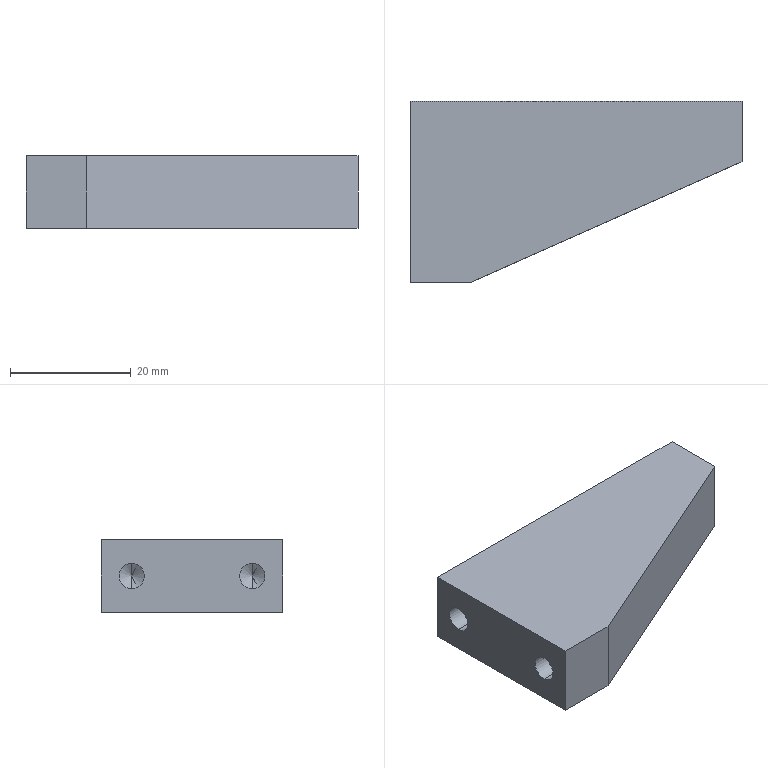Part | SolidWorks | features 3DProfileFeature 2, HoleWzd 2, Extrusion 1 | 1 solid | 23 faces | box 55 x 30 x 12 mm | volume 13823 mm3 | cylinder 8 | cone 8 | plane 7 | commonest cylinder face diameters 4.2 x8
STEP:
#1=CARTESIAN_POINT('',(-30.107,9.119,3.9));
#2=VERTEX_POINT('',#1);
#3=CARTESIAN_POINT('',(-30.107,9.119,8.1));
#4=VERTEX_POINT('',#3);
#5=CARTESIAN_POINT('',(-30.107,9.119,6.));
#6=DIRECTION('',(-1.,0.,0.));
#7=DIRECTION('',(0.,0.,1.));
#8=AXIS2_PLACEMENT_3D('',#5,#6,#7);
#9=CIRCLE('',#8,2.1);
#10=EDGE_CURVE('',#2,#4,#9,.T.);
#11=ORIENTED_EDGE('',*,*,#10,.F.);
#12=CARTESIAN_POINT('',(-40.107,9.119,3.9));
#13=VERTEX_POINT('',#12);
#14=CARTESIAN_POINT('',(-40.107,9.119,3.9));
#15=DIRECTION('',(-1.,0.,0.));
#16=VECTOR('',#15,1000.);
#17=LINE('',#14,#16);
#18=EDGE_CURVE('',#2,#13,#17,.T.);
#19=ORIENTED_EDGE('',*,*,#18,.T.);
#20=CARTESIAN_POINT('',(-40.107,9.119,8.1));
#21=VERTEX_POINT('',#20);
#22=CARTESIAN_POINT('',(-40.107,9.119,6.));
#23=DIRECTION('',(-1.,0.,0.));
#24=DIRECTION('',(0.,0.,1.));
#25=AXIS2_PLACEMENT_3D('',#22,#23,#24);
#26=CIRCLE('',#25,2.1);
#27=EDGE_CURVE('',#13,#21,#26,.T.);
#28=ORIENTED_EDGE('',*,*,#27,.T.);
#29=CARTESIAN_POINT('',(-40.107,9.119,8.1));
#30=DIRECTION('',(-1.,0.,0.));
#31=VECTOR('',#30,1000.);
#32=LINE('',#29,#31);
#33=EDGE_CURVE('',#4,#21,#32,.T.);
#34=ORIENTED_EDGE('',*,*,#33,.F.);
#35=EDGE_LOOP('',(#11,#19,#28,#34));
#36=FACE_OUTER_BOUND('',#35,.T.);
#37=CARTESIAN_POINT('',(-40.107,9.119,6.));
#38=DIRECTION('',(-1.,0.,0.));
#39=DIRECTION('',(0.,0.,1.));
#40=AXIS2_PLACEMENT_3D('',#37,#38,#39);
#41=CYLINDRICAL_SURFACE('',#40,2.1);
#42=ADVANCED_FACE('',(#36),#41,.F.);
#43=CARTESIAN_POINT('',(-28.845,9.119,6.));
#44=VERTEX_POINT('',#43);
#45=CARTESIAN_POINT('',(-30.107,9.119,8.1));
#46=DIRECTION('',(-0.515,0.,0.8572));
#47=VECTOR('',#46,1000.);
#48=LINE('',#45,#47);
#49=EDGE_CURVE('',#44,#4,#48,.T.);
#50=ORIENTED_EDGE('',*,*,#49,.F.);
#51=CARTESIAN_POINT('',(-30.107,9.119,3.9));
#52=DIRECTION('',(-0.515,0.,-0.8572));
#53=VECTOR('',#52,1000.);
#54=LINE('',#51,#53);
#55=EDGE_CURVE('',#44,#2,#54,.T.);
#56=ORIENTED_EDGE('',*,*,#55,.T.);
#57=ORIENTED_EDGE('',*,*,#10,.T.);
#58=EDGE_LOOP('',(#50,#56,#57));
#59=FACE_OUTER_BOUND('',#58,.T.);
#60=CARTESIAN_POINT('',(-30.107,9.119,6.));
#61=DIRECTION('',(-1.,0.,0.));
#62=DIRECTION('',(0.,0.,1.));
#63=AXIS2_PLACEMENT_3D('',#60,#61,#62);
#64=CONICAL_SURFACE('',#63,2.1,1.03);
#65=ADVANCED_FACE('',(#59),#64,.F.);
#66=CARTESIAN_POINT('',(-30.107,29.119,3.9));
#67=VERTEX_POINT('',#66);
#68=CARTESIAN_POINT('',(-30.107,29.119,8.1));
#69=VERTEX_POINT('',#68);
#70=CARTESIAN_POINT('',(-30.107,29.119,6.));
#71=DIRECTION('',(-1.,0.,0.));
#72=DIRECTION('',(0.,0.,1.));
#73=AXIS2_PLACEMENT_3D('',#70,#71,#72);
#74=CIRCLE('',#73,2.1);
#75=EDGE_CURVE('',#67,#69,#74,.T.);
#76=ORIENTED_EDGE('',*,*,#75,.F.);
#77=CARTESIAN_POINT('',(-40.107,29.119,3.9));
#78=VERTEX_POINT('',#77);
#79=CARTESIAN_POINT('',(-40.107,29.119,3.9));
#80=DIRECTION('',(-1.,0.,0.));
#81=VECTOR('',#80,1000.);
#82=LINE('',#79,#81);
#83=EDGE_CURVE('',#67,#78,#82,.T.);
#84=ORIENTED_EDGE('',*,*,#83,.T.);
#85=CARTESIAN_POINT('',(-40.107,29.119,8.1));
#86=VERTEX_POINT('',#85);
#87=CARTESIAN_POINT('',(-40.107,29.119,6.));
#88=DIRECTION('',(-1.,0.,0.));
#89=DIRECTION('',(0.,0.,1.));
#90=AXIS2_PLACEMENT_3D('',#87,#88,#89);
#91=CIRCLE('',#90,2.1);
#92=EDGE_CURVE('',#78,#86,#91,.T.);
#93=ORIENTED_EDGE('',*,*,#92,.T.);
#94=CARTESIAN_POINT('',(-40.107,29.119,8.1));
#95=DIRECTION('',(-1.,0.,0.));
#96=VECTOR('',#95,1000.);
#97=LINE('',#94,#96);
#98=EDGE_CURVE('',#69,#86,#97,.T.);
#99=ORIENTED_EDGE('',*,*,#98,.F.);
#100=EDGE_LOOP('',(#76,#84,#93,#99));
#101=FACE_OUTER_BOUND('',#100,.T.);
#102=CARTESIAN_POINT('',(-40.107,29.119,6.));
#103=DIRECTION('',(-1.,0.,0.));
#104=DIRECTION('',(0.,0.,1.));
#105=AXIS2_PLACEMENT_3D('',#102,#103,#104);
#106=CYLINDRICAL_SURFACE('',#105,2.1);
#107=ADVANCED_FACE('',(#101),#106,.F.);
#108=CARTESIAN_POINT('',(-28.845,29.119,6.));
#109=VERTEX_POINT('',#108);
#110=CARTESIAN_POINT('',(-30.107,29.119,8.1));
#111=DIRECTION('',(-0.515,0.,0.8572));
#112=VECTOR('',#111,1000.);
#113=LINE('',#110,#112);
#114=EDGE_CURVE('',#109,#69,#113,.T.);
#115=ORIENTED_EDGE('',*,*,#114,.F.);
#116=CARTESIAN_POINT('',(-30.107,29.119,3.9));
#117=DIRECTION('',(-0.515,0.,-0.8572));
#118=VECTOR('',#117,1000.);
#119=LINE('',#116,#118);
#120=EDGE_CURVE('',#109,#67,#119,.T.);
#121=ORIENTED_EDGE('',*,*,#120,.T.);
#122=ORIENTED_EDGE('',*,*,#75,.T.);
#123=EDGE_LOOP('',(#115,#121,#122));
#124=FACE_OUTER_BOUND('',#123,.T.);
#125=CARTESIAN_POINT('',(-30.107,29.119,6.));
#126=DIRECTION('',(-1.,0.,0.));
#127=DIRECTION('',(0.,0.,1.));
#128=AXIS2_PLACEMENT_3D('',#125,#126,#127);
#129=CONICAL_SURFACE('',#128,2.1,1.03);
#130=ADVANCED_FACE('',(#124),#129,.F.);
#131=CARTESIAN_POINT('',(-24.107,24.119,3.9));
#132=VERTEX_POINT('',#131);
#133=CARTESIAN_POINT('',(-24.107,24.119,8.1));
#134=VERTEX_POINT('',#133);
#135=CARTESIAN_POINT('',(-24.107,24.119,6.));
#136=DIRECTION('',(0.,1.,0.));
#137=DIRECTION('',(0.,0.,1.));
#138=AXIS2_PLACEMENT_3D('',#135,#136,#137);
#139=CIRCLE('',#138,2.1);
#140=EDGE_CURVE('',#132,#134,#139,.T.);
#141=ORIENTED_EDGE('',*,*,#140,.F.);
#142=CARTESIAN_POINT('',(-24.107,34.119,3.9));
#143=VERTEX_POINT('',#142);
#144=CARTESIAN_POINT('',(-24.107,34.119,3.9));
#145=DIRECTION('',(0.,1.,0.));
#146=VECTOR('',#145,1000.);
#147=LINE('',#144,#146);
#148=EDGE_CURVE('',#132,#143,#147,.T.);
#149=ORIENTED_EDGE('',*,*,#148,.T.);
#150=CARTESIAN_POINT('',(-24.107,34.119,8.1));
#151=VERTEX_POINT('',#150);
#152=CARTESIAN_POINT('',(-24.107,34.119,6.));
#153=DIRECTION('',(0.,1.,0.));
#154=DIRECTION('',(0.,0.,1.));
#155=AXIS2_PLACEMENT_3D('',#152,#153,#154);
#156=CIRCLE('',#155,2.1);
#157=EDGE_CURVE('',#143,#151,#156,.T.);
#158=ORIENTED_EDGE('',*,*,#157,.T.);
#159=CARTESIAN_POINT('',(-24.107,34.119,8.1));
#160=DIRECTION('',(0.,1.,0.));
#161=VECTOR('',#160,1000.);
#162=LINE('',#159,#161);
#163=EDGE_CURVE('',#134,#151,#162,.T.);
#164=ORIENTED_EDGE('',*,*,#163,.F.);
#165=EDGE_LOOP('',(#141,#149,#158,#164));
#166=FACE_OUTER_BOUND('',#165,.T.);
#167=CARTESIAN_POINT('',(-24.107,34.119,6.));
#168=DIRECTION('',(0.,1.,0.));
#169=DIRECTION('',(0.,0.,1.));
#170=AXIS2_PLACEMENT_3D('',#167,#168,#169);
#171=CYLINDRICAL_SURFACE('',#170,2.1);
#172=ADVANCED_FACE('',(#166),#171,.F.);
#173=CARTESIAN_POINT('',(-24.107,22.857,6.));
#174=VERTEX_POINT('',#173);
#175=CARTESIAN_POINT('',(-24.107,24.119,8.1));
#176=DIRECTION('',(0.,0.515,0.8572));
#177=VECTOR('',#176,1000.);
#178=LINE('',#175,#177);
#179=EDGE_CURVE('',#174,#134,#178,.T.);
#180=ORIENTED_EDGE('',*,*,#179,.F.);
#181=CARTESIAN_POINT('',(-24.107,24.119,3.9));
#182=DIRECTION('',(0.,0.515,-0.8572));
#183=VECTOR('',#182,1000.);
#184=LINE('',#181,#183);
#185=EDGE_CURVE('',#174,#132,#184,.T.);
#186=ORIENTED_EDGE('',*,*,#185,.T.);
#187=ORIENTED_EDGE('',*,*,#140,.T.);
#188=EDGE_LOOP('',(#180,#186,#187));
#189=FACE_OUTER_BOUND('',#188,.T.);
#190=CARTESIAN_POINT('',(-24.107,24.119,6.));
#191=DIRECTION('',(0.,1.,0.));
#192=DIRECTION('',(0.,0.,1.));
#193=AXIS2_PLACEMENT_3D('',#190,#191,#192);
#194=CONICAL_SURFACE('',#193,2.1,1.03);
#195=ADVANCED_FACE('',(#189),#194,.F.);
#196=CARTESIAN_POINT('',(5.893,24.119,3.9));
#197=VERTEX_POINT('',#196);
#198=CARTESIAN_POINT('',(5.893,24.119,8.1));
#199=VERTEX_POINT('',#198);
#200=CARTESIAN_POINT('',(5.893,24.119,6.));
#201=DIRECTION('',(0.,1.,0.));
#202=DIRECTION('',(0.,0.,1.));
#203=AXIS2_PLACEMENT_3D('',#200,#201,#202);
#204=CIRCLE('',#203,2.1);
#205=EDGE_CURVE('',#197,#199,#204,.T.);
#206=ORIENTED_EDGE('',*,*,#205,.F.);
#207=CARTESIAN_POINT('',(5.893,34.119,3.9));
#208=VERTEX_POINT('',#207);
#209=CARTESIAN_POINT('',(5.893,34.119,3.9));
#210=DIRECTION('',(0.,1.,0.));
#211=VECTOR('',#210,1000.);
#212=LINE('',#209,#211);
#213=EDGE_CURVE('',#197,#208,#212,.T.);
#214=ORIENTED_EDGE('',*,*,#213,.T.);
#215=CARTESIAN_POINT('',(5.893,34.119,8.1));
#216=VERTEX_POINT('',#215);
#217=CARTESIAN_POINT('',(5.893,34.119,6.));
#218=DIRECTION('',(0.,1.,0.));
#219=DIRECTION('',(0.,0.,1.));
#220=AXIS2_PLACEMENT_3D('',#217,#218,#219);
#221=CIRCLE('',#220,2.1);
#222=EDGE_CURVE('',#208,#216,#221,.T.);
#223=ORIENTED_EDGE('',*,*,#222,.T.);
#224=CARTESIAN_POINT('',(5.893,34.119,8.1));
#225=DIRECTION('',(0.,1.,0.));
#226=VECTOR('',#225,1000.);
#227=LINE('',#224,#226);
#228=EDGE_CURVE('',#199,#216,#227,.T.);
#229=ORIENTED_EDGE('',*,*,#228,.F.);
#230=EDGE_LOOP('',(#206,#214,#223,#229));
#231=FACE_OUTER_BOUND('',#230,.T.);
#232=CARTESIAN_POINT('',(5.893,34.119,6.));
#233=DIRECTION('',(0.,1.,0.));
#234=DIRECTION('',(0.,0.,1.));
#235=AXIS2_PLACEMENT_3D('',#232,#233,#234);
#236=CYLINDRICAL_SURFACE('',#235,2.1);
#237=ADVANCED_FACE('',(#231),#236,.F.);
#238=CARTESIAN_POINT('',(5.893,22.857,6.));
#239=VERTEX_POINT('',#238);
#240=CARTESIAN_POINT('',(5.893,24.119,8.1));
#241=DIRECTION('',(0.,0.515,0.8572));
#242=VECTOR('',#241,1000.);
#243=LINE('',#240,#242);
#244=EDGE_CURVE('',#239,#199,#243,.T.);
#245=ORIENTED_EDGE('',*,*,#244,.F.);
#246=CARTESIAN_POINT('',(5.893,24.119,3.9));
#247=DIRECTION('',(0.,0.515,-0.8572));
#248=VECTOR('',#247,1000.);
#249=LINE('',#246,#248);
#250=EDGE_CURVE('',#239,#197,#249,.T.);
#251=ORIENTED_EDGE('',*,*,#250,.T.);
#252=ORIENTED_EDGE('',*,*,#205,.T.);
#253=EDGE_LOOP('',(#245,#251,#252));
#254=FACE_OUTER_BOUND('',#253,.T.);
#255=CARTESIAN_POINT('',(5.893,24.119,6.));
#256=DIRECTION('',(0.,1.,0.));
#257=DIRECTION('',(0.,0.,1.));
#258=AXIS2_PLACEMENT_3D('',#255,#256,#257);
#259=CONICAL_SURFACE('',#258,2.1,1.03);
#260=ADVANCED_FACE('',(#254),#259,.F.);
#261=CARTESIAN_POINT('',(-30.107,4.119,0.));
#262=VERTEX_POINT('',#261);
#263=CARTESIAN_POINT('',(14.893,24.119,0.));
#264=VERTEX_POINT('',#263);
#265=CARTESIAN_POINT('',(14.893,24.119,0.));
#266=DIRECTION('',(0.9138,0.4061,0.));
#267=VECTOR('',#266,1000.);
#268=LINE('',#265,#267);
#269=EDGE_CURVE('',#262,#264,#268,.T.);
#270=ORIENTED_EDGE('',*,*,#269,.T.);
#271=CARTESIAN_POINT('',(14.893,24.119,12.));
#272=VERTEX_POINT('',#271);
#273=CARTESIAN_POINT('',(14.893,24.119,12.));
#274=DIRECTION('',(0.,0.,-1.));
#275=VECTOR('',#274,1000.);
#276=LINE('',#273,#275);
#277=EDGE_CURVE('',#272,#264,#276,.T.);
#278=ORIENTED_EDGE('',*,*,#277,.F.);
#279=CARTESIAN_POINT('',(-30.107,4.119,12.));
#280=VERTEX_POINT('',#279);
#281=CARTESIAN_POINT('',(14.893,24.119,12.));
#282=DIRECTION('',(0.9138,0.4061,0.));
#283=VECTOR('',#282,1000.);
#284=LINE('',#281,#283);
#285=EDGE_CURVE('',#280,#272,#284,.T.);
#286=ORIENTED_EDGE('',*,*,#285,.F.);
#287=CARTESIAN_POINT('',(-30.107,4.119,12.));
#288=DIRECTION('',(0.,0.,-1.));
#289=VECTOR('',#288,1000.);
#290=LINE('',#287,#289);
#291=EDGE_CURVE('',#280,#262,#290,.T.);
#292=ORIENTED_EDGE('',*,*,#291,.T.);
#293=EDGE_LOOP('',(#270,#278,#286,#292));
#294=FACE_OUTER_BOUND('',#293,.T.);
#295=CARTESIAN_POINT('',(14.893,24.119,12.));
#296=DIRECTION('',(-0.4061,0.9138,0.));
#297=DIRECTION('',(-0.9138,-0.4061,0.));
#298=AXIS2_PLACEMENT_3D('',#295,#296,#297);
#299=PLANE('',#298);
#300=ADVANCED_FACE('',(#294),#299,.F.);
#301=CARTESIAN_POINT('',(14.893,34.119,0.));
#302=VERTEX_POINT('',#301);
#303=CARTESIAN_POINT('',(14.893,34.119,0.));
#304=DIRECTION('',(0.,1.,0.));
#305=VECTOR('',#304,1000.);
#306=LINE('',#303,#305);
#307=EDGE_CURVE('',#264,#302,#306,.T.);
#308=ORIENTED_EDGE('',*,*,#307,.T.);
#309=CARTESIAN_POINT('',(14.893,34.119,12.));
#310=VERTEX_POINT('',#309);
#311=CARTESIAN_POINT('',(14.893,34.119,12.));
#312=DIRECTION('',(0.,0.,-1.));
#313=VECTOR('',#312,1000.);
#314=LINE('',#311,#313);
#315=EDGE_CURVE('',#310,#302,#314,.T.);
#316=ORIENTED_EDGE('',*,*,#315,.F.);
#317=CARTESIAN_POINT('',(14.893,34.119,12.));
#318=DIRECTION('',(0.,1.,0.));
#319=VECTOR('',#318,1000.);
#320=LINE('',#317,#319);
#321=EDGE_CURVE('',#272,#310,#320,.T.);
#322=ORIENTED_EDGE('',*,*,#321,.F.);
#323=ORIENTED_EDGE('',*,*,#277,.T.);
#324=EDGE_LOOP('',(#308,#316,#322,#323));
#325=FACE_OUTER_BOUND('',#324,.T.);
#326=CARTESIAN_POINT('',(14.893,34.119,12.));
#327=DIRECTION('',(-1.,0.,0.));
#328=DIRECTION('',(0.,-1.,0.));
#329=AXIS2_PLACEMENT_3D('',#326,#327,#328);
#330=PLANE('',#329);
#331=ADVANCED_FACE('',(#325),#330,.F.);
#332=CARTESIAN_POINT('',(-24.107,34.119,6.));
#333=DIRECTION('',(0.,1.,0.));
#334=DIRECTION('',(0.,0.,1.));
#335=AXIS2_PLACEMENT_3D('',#332,#333,#334);
#336=CIRCLE('',#335,2.1);
#337=EDGE_CURVE('',#151,#143,#336,.T.);
#338=ORIENTED_EDGE('',*,*,#337,.F.);
#339=ORIENTED_EDGE('',*,*,#157,.F.);
#340=EDGE_LOOP('',(#338,#339));
#341=FACE_BOUND('',#340,.T.);
#342=CARTESIAN_POINT('',(5.893,34.119,6.));
#343=DIRECTION('',(0.,1.,0.));
#344=DIRECTION('',(0.,0.,1.));
#345=AXIS2_PLACEMENT_3D('',#342,#343,#344);
#346=CIRCLE('',#345,2.1);
#347=EDGE_CURVE('',#216,#208,#346,.T.);
#348=ORIENTED_EDGE('',*,*,#347,.F.);
#349=ORIENTED_EDGE('',*,*,#222,.F.);
#350=EDGE_LOOP('',(#348,#349));
#351=FACE_BOUND('',#350,.T.);
#352=CARTESIAN_POINT('',(-40.107,34.119,0.));
#353=VERTEX_POINT('',#352);
#354=CARTESIAN_POINT('',(-40.107,34.119,0.));
#355=DIRECTION('',(-1.,0.,0.));
#356=VECTOR('',#355,1000.);
#357=LINE('',#354,#356);
#358=EDGE_CURVE('',#302,#353,#357,.T.);
#359=ORIENTED_EDGE('',*,*,#358,.T.);
#360=CARTESIAN_POINT('',(-40.107,34.119,12.));
#361=VERTEX_POINT('',#360);
#362=CARTESIAN_POINT('',(-40.107,34.119,12.));
#363=DIRECTION('',(0.,0.,-1.));
#364=VECTOR('',#363,1000.);
#365=LINE('',#362,#364);
#366=EDGE_CURVE('',#361,#353,#365,.T.);
#367=ORIENTED_EDGE('',*,*,#366,.F.);
#368=CARTESIAN_POINT('',(-40.107,34.119,12.));
#369=DIRECTION('',(-1.,0.,0.));
#370=VECTOR('',#369,1000.);
#371=LINE('',#368,#370);
#372=EDGE_CURVE('',#310,#361,#371,.T.);
#373=ORIENTED_EDGE('',*,*,#372,.F.);
#374=ORIENTED_EDGE('',*,*,#315,.T.);
#375=EDGE_LOOP('',(#359,#367,#373,#374));
#376=FACE_OUTER_BOUND('',#375,.T.);
#377=CARTESIAN_POINT('',(-40.107,34.119,12.));
#378=DIRECTION('',(0.,-1.,0.));
#379=DIRECTION('',(0.,0.,-1.));
#380=AXIS2_PLACEMENT_3D('',#377,#378,#379);
#381=PLANE('',#380);
#382=ADVANCED_FACE('',(#341,#351,#376),#381,.F.);
#383=CARTESIAN_POINT('',(-40.107,9.119,6.));
#384=DIRECTION('',(-1.,0.,0.));
#385=DIRECTION('',(0.,0.,1.));
#386=AXIS2_PLACEMENT_3D('',#383,#384,#385);
#387=CIRCLE('',#386,2.1);
#388=EDGE_CURVE('',#21,#13,#387,.T.);
#389=ORIENTED_EDGE('',*,*,#388,.F.);
#390=ORIENTED_EDGE('',*,*,#27,.F.);
#391=EDGE_LOOP('',(#389,#390));
#392=FACE_BOUND('',#391,.T.);
#393=CARTESIAN_POINT('',(-40.107,29.119,6.));
#394=DIRECTION('',(-1.,0.,0.));
#395=DIRECTION('',(0.,0.,1.));
#396=AXIS2_PLACEMENT_3D('',#393,#394,#395);
#397=CIRCLE('',#396,2.1);
#398=EDGE_CURVE('',#86,#78,#397,.T.);
#399=ORIENTED_EDGE('',*,*,#398,.F.);
#400=ORIENTED_EDGE('',*,*,#92,.F.);
#401=EDGE_LOOP('',(#399,#400));
#402=FACE_BOUND('',#401,.T.);
#403=CARTESIAN_POINT('',(-40.107,4.119,0.));
#404=VERTEX_POINT('',#403);
#405=CARTESIAN_POINT('',(-40.107,4.119,0.));
#406=DIRECTION('',(0.,-1.,0.));
#407=VECTOR('',#406,1000.);
#408=LINE('',#405,#407);
#409=EDGE_CURVE('',#353,#404,#408,.T.);
#410=ORIENTED_EDGE('',*,*,#409,.T.);
#411=CARTESIAN_POINT('',(-40.107,4.119,12.));
#412=VERTEX_POINT('',#411);
#413=CARTESIAN_POINT('',(-40.107,4.119,12.));
#414=DIRECTION('',(0.,0.,-1.));
#415=VECTOR('',#414,1000.);
#416=LINE('',#413,#415);
#417=EDGE_CURVE('',#412,#404,#416,.T.);
#418=ORIENTED_EDGE('',*,*,#417,.F.);
#419=CARTESIAN_POINT('',(-40.107,4.119,12.));
#420=DIRECTION('',(0.,-1.,0.));
#421=VECTOR('',#420,1000.);
#422=LINE('',#419,#421);
#423=EDGE_CURVE('',#361,#412,#422,.T.);
#424=ORIENTED_EDGE('',*,*,#423,.F.);
#425=ORIENTED_EDGE('',*,*,#366,.T.);
#426=EDGE_LOOP('',(#410,#418,#424,#425));
#427=FACE_OUTER_BOUND('',#426,.T.);
#428=CARTESIAN_POINT('',(-40.107,4.119,12.));
#429=DIRECTION('',(1.,0.,0.));
#430=DIRECTION('',(0.,0.,-1.));
#431=AXIS2_PLACEMENT_3D('',#428,#429,#430);
#432=PLANE('',#431);
#433=ADVANCED_FACE('',(#392,#402,#427),#432,.F.);
#434=CARTESIAN_POINT('',(-30.107,4.119,0.));
#435=DIRECTION('',(1.,0.,0.));
#436=VECTOR('',#435,1000.);
#437=LINE('',#434,#436);
#438=EDGE_CURVE('',#404,#262,#437,.T.);
#439=ORIENTED_EDGE('',*,*,#438,.T.);
#440=ORIENTED_EDGE('',*,*,#291,.F.);
#441=CARTESIAN_POINT('',(-30.107,4.119,12.));
#442=DIRECTION('',(1.,0.,0.));
#443=VECTOR('',#442,1000.);
#444=LINE('',#441,#443);
#445=EDGE_CURVE('',#412,#280,#444,.T.);
#446=ORIENTED_EDGE('',*,*,#445,.F.);
#447=ORIENTED_EDGE('',*,*,#417,.T.);
#448=EDGE_LOOP('',(#439,#440,#446,#447));
#449=FACE_OUTER_BOUND('',#448,.T.);
#450=CARTESIAN_POINT('',(-30.107,4.119,12.));
#451=DIRECTION('',(0.,1.,0.));
#452=DIRECTION('',(-1.,0.,0.));
#453=AXIS2_PLACEMENT_3D('',#450,#451,#452);
#454=PLANE('',#453);
#455=ADVANCED_FACE('',(#449),#454,.F.);
#456=ORIENTED_EDGE('',*,*,#285,.T.);
#457=ORIENTED_EDGE('',*,*,#321,.T.);
#458=ORIENTED_EDGE('',*,*,#372,.T.);
#459=ORIENTED_EDGE('',*,*,#423,.T.);
#460=ORIENTED_EDGE('',*,*,#445,.T.);
#461=EDGE_LOOP('',(#456,#457,#458,#459,#460));
#462=FACE_OUTER_BOUND('',#461,.T.);
#463=CARTESIAN_POINT('',(-40.107,-0.3259,12.));
#464=DIRECTION('',(0.,0.,-1.));
#465=DIRECTION('',(-1.,0.,0.));
#466=AXIS2_PLACEMENT_3D('',#463,#464,#465);
#467=PLANE('',#466);
#468=ADVANCED_FACE('',(#462),#467,.F.);
#469=ORIENTED_EDGE('',*,*,#269,.F.);
#470=ORIENTED_EDGE('',*,*,#438,.F.);
#471=ORIENTED_EDGE('',*,*,#409,.F.);
#472=ORIENTED_EDGE('',*,*,#358,.F.);
#473=ORIENTED_EDGE('',*,*,#307,.F.);
#474=EDGE_LOOP('',(#469,#470,#471,#472,#473));
#475=FACE_OUTER_BOUND('',#474,.T.);
#476=CARTESIAN_POINT('',(-40.107,-0.3259,0.));
#477=DIRECTION('',(0.,0.,-1.));
#478=DIRECTION('',(-1.,0.,0.));
#479=AXIS2_PLACEMENT_3D('',#476,#477,#478);
#480=PLANE('',#479);
#481=ADVANCED_FACE('',(#475),#480,.T.);
#482=ORIENTED_EDGE('',*,*,#250,.F.);
#483=ORIENTED_EDGE('',*,*,#244,.T.);
#484=CARTESIAN_POINT('',(5.893,24.119,6.));
#485=DIRECTION('',(0.,1.,0.));
#486=DIRECTION('',(0.,0.,1.));
#487=AXIS2_PLACEMENT_3D('',#484,#485,#486);
#488=CIRCLE('',#487,2.1);
#489=EDGE_CURVE('',#199,#197,#488,.T.);
#490=ORIENTED_EDGE('',*,*,#489,.T.);
#491=EDGE_LOOP('',(#482,#483,#490));
#492=FACE_OUTER_BOUND('',#491,.T.);
#493=CARTESIAN_POINT('',(5.893,24.119,6.));
#494=DIRECTION('',(0.,1.,0.));
#495=DIRECTION('',(0.,0.,1.));
#496=AXIS2_PLACEMENT_3D('',#493,#494,#495);
#497=CONICAL_SURFACE('',#496,2.1,1.03);
#498=ADVANCED_FACE('',(#492),#497,.F.);
#499=ORIENTED_EDGE('',*,*,#213,.F.);
#500=ORIENTED_EDGE('',*,*,#489,.F.);
#501=ORIENTED_EDGE('',*,*,#228,.T.);
#502=ORIENTED_EDGE('',*,*,#347,.T.);
#503=EDGE_LOOP('',(#499,#500,#501,#502));
#504=FACE_OUTER_BOUND('',#503,.T.);
#505=CARTESIAN_POINT('',(5.893,34.119,6.));
#506=DIRECTION('',(0.,1.,0.));
#507=DIRECTION('',(0.,0.,1.));
#508=AXIS2_PLACEMENT_3D('',#505,#506,#507);
#509=CYLINDRICAL_SURFACE('',#508,2.1);
#510=ADVANCED_FACE('',(#504),#509,.F.);
#511=ORIENTED_EDGE('',*,*,#185,.F.);
#512=ORIENTED_EDGE('',*,*,#179,.T.);
#513=CARTESIAN_POINT('',(-24.107,24.119,6.));
#514=DIRECTION('',(0.,1.,0.));
#515=DIRECTION('',(0.,0.,1.));
#516=AXIS2_PLACEMENT_3D('',#513,#514,#515);
#517=CIRCLE('',#516,2.1);
#518=EDGE_CURVE('',#134,#132,#517,.T.);
#519=ORIENTED_EDGE('',*,*,#518,.T.);
#520=EDGE_LOOP('',(#511,#512,#519));
#521=FACE_OUTER_BOUND('',#520,.T.);
#522=CARTESIAN_POINT('',(-24.107,24.119,6.));
#523=DIRECTION('',(0.,1.,0.));
#524=DIRECTION('',(0.,0.,1.));
#525=AXIS2_PLACEMENT_3D('',#522,#523,#524);
#526=CONICAL_SURFACE('',#525,2.1,1.03);
#527=ADVANCED_FACE('',(#521),#526,.F.);
#528=ORIENTED_EDGE('',*,*,#148,.F.);
#529=ORIENTED_EDGE('',*,*,#518,.F.);
#530=ORIENTED_EDGE('',*,*,#163,.T.);
#531=ORIENTED_EDGE('',*,*,#337,.T.);
#532=EDGE_LOOP('',(#528,#529,#530,#531));
#533=FACE_OUTER_BOUND('',#532,.T.);
#534=CARTESIAN_POINT('',(-24.107,34.119,6.));
#535=DIRECTION('',(0.,1.,0.));
#536=DIRECTION('',(0.,0.,1.));
#537=AXIS2_PLACEMENT_3D('',#534,#535,#536);
#538=CYLINDRICAL_SURFACE('',#537,2.1);
#539=ADVANCED_FACE('',(#533),#538,.F.);
#540=ORIENTED_EDGE('',*,*,#120,.F.);
#541=ORIENTED_EDGE('',*,*,#114,.T.);
#542=CARTESIAN_POINT('',(-30.107,29.119,6.));
#543=DIRECTION('',(-1.,0.,0.));
#544=DIRECTION('',(0.,0.,1.));
#545=AXIS2_PLACEMENT_3D('',#542,#543,#544);
#546=CIRCLE('',#545,2.1);
#547=EDGE_CURVE('',#69,#67,#546,.T.);
#548=ORIENTED_EDGE('',*,*,#547,.T.);
#549=EDGE_LOOP('',(#540,#541,#548));
#550=FACE_OUTER_BOUND('',#549,.T.);
#551=CARTESIAN_POINT('',(-30.107,29.119,6.));
#552=DIRECTION('',(-1.,0.,0.));
#553=DIRECTION('',(0.,0.,1.));
#554=AXIS2_PLACEMENT_3D('',#551,#552,#553);
#555=CONICAL_SURFACE('',#554,2.1,1.03);
#556=ADVANCED_FACE('',(#550),#555,.F.);
#557=ORIENTED_EDGE('',*,*,#83,.F.);
#558=ORIENTED_EDGE('',*,*,#547,.F.);
#559=ORIENTED_EDGE('',*,*,#98,.T.);
#560=ORIENTED_EDGE('',*,*,#398,.T.);
#561=EDGE_LOOP('',(#557,#558,#559,#560));
#562=FACE_OUTER_BOUND('',#561,.T.);
#563=CARTESIAN_POINT('',(-40.107,29.119,6.));
#564=DIRECTION('',(-1.,0.,0.));
#565=DIRECTION('',(0.,0.,1.));
#566=AXIS2_PLACEMENT_3D('',#563,#564,#565);
#567=CYLINDRICAL_SURFACE('',#566,2.1);
#568=ADVANCED_FACE('',(#562),#567,.F.);
#569=ORIENTED_EDGE('',*,*,#55,.F.);
#570=ORIENTED_EDGE('',*,*,#49,.T.);
#571=CARTESIAN_POINT('',(-30.107,9.119,6.));
#572=DIRECTION('',(-1.,0.,0.));
#573=DIRECTION('',(0.,0.,1.));
#574=AXIS2_PLACEMENT_3D('',#571,#572,#573);
#575=CIRCLE('',#574,2.1);
#576=EDGE_CURVE('',#4,#2,#575,.T.);
#577=ORIENTED_EDGE('',*,*,#576,.T.);
#578=EDGE_LOOP('',(#569,#570,#577));
#579=FACE_OUTER_BOUND('',#578,.T.);
#580=CARTESIAN_POINT('',(-30.107,9.119,6.));
#581=DIRECTION('',(-1.,0.,0.));
#582=DIRECTION('',(0.,0.,1.));
#583=AXIS2_PLACEMENT_3D('',#580,#581,#582);
#584=CONICAL_SURFACE('',#583,2.1,1.03);
#585=ADVANCED_FACE('',(#579),#584,.F.);
#586=ORIENTED_EDGE('',*,*,#18,.F.);
#587=ORIENTED_EDGE('',*,*,#576,.F.);
#588=ORIENTED_EDGE('',*,*,#33,.T.);
#589=ORIENTED_EDGE('',*,*,#388,.T.);
#590=EDGE_LOOP('',(#586,#587,#588,#589));
#591=FACE_OUTER_BOUND('',#590,.T.);
#592=CARTESIAN_POINT('',(-40.107,9.119,6.));
#593=DIRECTION('',(-1.,0.,0.));
#594=DIRECTION('',(0.,0.,1.));
#595=AXIS2_PLACEMENT_3D('',#592,#593,#594);
#596=CYLINDRICAL_SURFACE('',#595,2.1);
#597=ADVANCED_FACE('',(#591),#596,.F.);
#598=CLOSED_SHELL('',(#42,#65,#107,#130,#172,#195,#237,#260,#300,#331,#382,#433,#455,#468,#481,#498,#510,#527,#539,#556,#568,#585,#597));
#599=MANIFOLD_SOLID_BREP('',#598);
#600=CARTESIAN_POINT('',(0.,0.,0.));
#601=DIRECTION('',(0.,0.,1.));
#602=DIRECTION('',(1.,0.,0.));
#603=AXIS2_PLACEMENT_3D('',#600,#601,#602);
#604=(LENGTH_UNIT()NAMED_UNIT(*)SI_UNIT(.MILLI.,.METRE.));
#605=UNCERTAINTY_MEASURE_WITH_UNIT(LENGTH_MEASURE(0.00001),#604,'','');
#606=(NAMED_UNIT(*)PLANE_ANGLE_UNIT()SI_UNIT($,.RADIAN.));
#607=(NAMED_UNIT(*)SI_UNIT($,.STERADIAN.)SOLID_ANGLE_UNIT());
#608=(GEOMETRIC_REPRESENTATION_CONTEXT(3)GLOBAL_UNCERTAINTY_ASSIGNED_CONTEXT((#605))GLOBAL_UNIT_ASSIGNED_CONTEXT((#604,#606,#607))REPRESENTATION_CONTEXT('',''));
#609=ADVANCED_BREP_SHAPE_REPRESENTATION('',(#599,#603),#608);